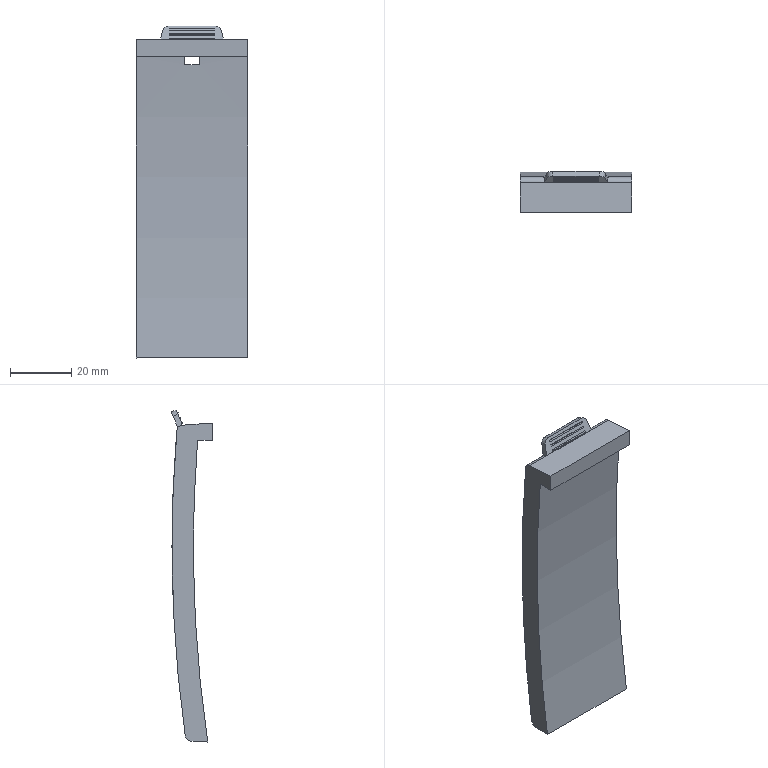Part | STEP file | ZXW735-L-95-03 | 1 solid | 151 faces | box 36.6 x 13.445 x 108.794 mm | volume 27625 mm3 | plane 92 | cylinder 59 | commonest cylinder face diameters 1.2 x32 892.889 x16 0.5 x4 4 x4 5.8 x1 879.489 x1